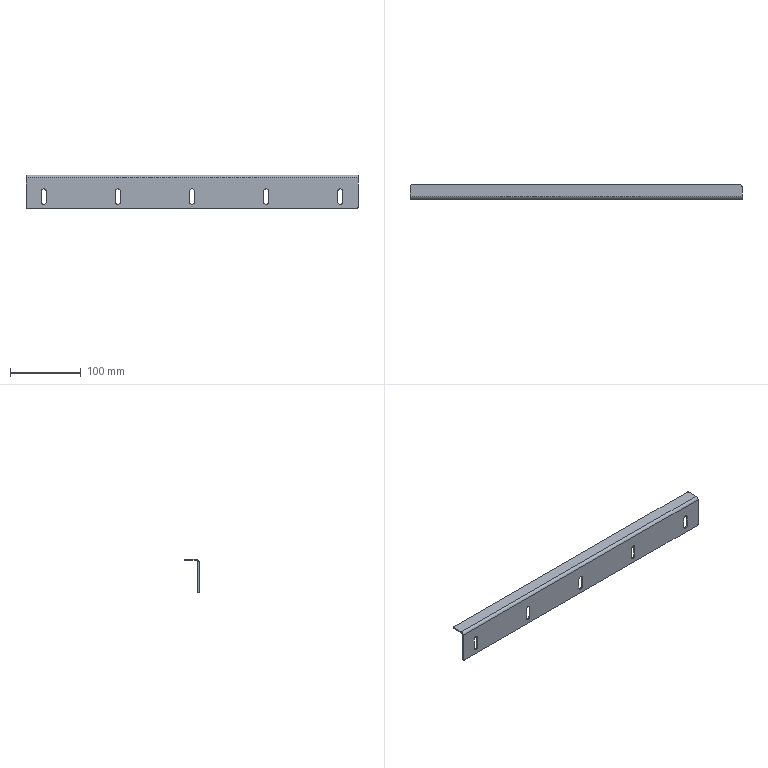Part | STEP file | 1 solid | 39 faces | box 470 x 20 x 48 mm | volume 59388 mm3 | cylinder 21 | plane 18 | commonest cylinder face diameters 7 x15 4 x5 8 x1